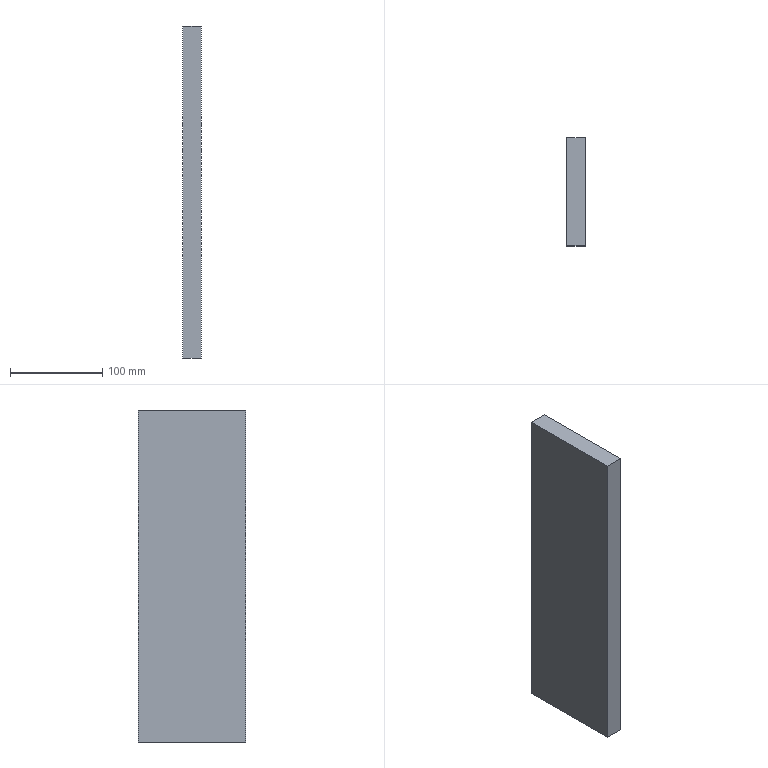Part | NX | features 底座(默认<按焊接>) 2 | 1 solid | 6 faces | box 20 x 116.68 x 360 mm | volume 840096 mm3 | plane 6
STEP:
#1=CARTESIAN_POINT('',(2704.525,684.,-26.));
#2=VERTEX_POINT('',#1);
#3=CARTESIAN_POINT('',(2704.525,567.32,-26.));
#4=VERTEX_POINT('',#3);
#5=CARTESIAN_POINT('',(2704.525,684.,-26.));
#6=DIRECTION('',(0.,-1.,0.));
#7=VECTOR('',#6,1000.);
#8=LINE('',#5,#7);
#9=EDGE_CURVE('',#2,#4,#8,.T.);
#10=ORIENTED_EDGE('',*,*,#9,.T.);
#11=CARTESIAN_POINT('',(2704.525,567.32,-386.));
#12=VERTEX_POINT('',#11);
#13=CARTESIAN_POINT('',(2704.525,567.32,-386.));
#14=DIRECTION('',(0.,0.,1.));
#15=VECTOR('',#14,1000.);
#16=LINE('',#13,#15);
#17=EDGE_CURVE('',#12,#4,#16,.T.);
#18=ORIENTED_EDGE('',*,*,#17,.F.);
#19=CARTESIAN_POINT('',(2704.525,684.,-386.));
#20=VERTEX_POINT('',#19);
#21=CARTESIAN_POINT('',(2704.525,684.,-386.));
#22=DIRECTION('',(0.,-1.,0.));
#23=VECTOR('',#22,1000.);
#24=LINE('',#21,#23);
#25=EDGE_CURVE('',#20,#12,#24,.T.);
#26=ORIENTED_EDGE('',*,*,#25,.F.);
#27=CARTESIAN_POINT('',(2704.525,684.,-386.));
#28=DIRECTION('',(0.,0.,1.));
#29=VECTOR('',#28,1000.);
#30=LINE('',#27,#29);
#31=EDGE_CURVE('',#20,#2,#30,.T.);
#32=ORIENTED_EDGE('',*,*,#31,.T.);
#33=EDGE_LOOP('',(#10,#18,#26,#32));
#34=FACE_BOUND('',#33,.T.);
#35=CARTESIAN_POINT('',(2704.525,684.,-386.));
#36=DIRECTION('',(-1.,0.,0.));
#37=DIRECTION('',(0.,0.,1.));
#38=AXIS2_PLACEMENT_3D('',#35,#36,#37);
#39=PLANE('',#38);
#40=ADVANCED_FACE('',(#34),#39,.F.);
#41=CARTESIAN_POINT('',(2684.525,567.32,-26.));
#42=VERTEX_POINT('',#41);
#43=CARTESIAN_POINT('',(2704.525,567.32,-26.));
#44=DIRECTION('',(-1.,0.,0.));
#45=VECTOR('',#44,1000.);
#46=LINE('',#43,#45);
#47=EDGE_CURVE('',#4,#42,#46,.T.);
#48=ORIENTED_EDGE('',*,*,#47,.T.);
#49=CARTESIAN_POINT('',(2684.525,567.32,-386.));
#50=VERTEX_POINT('',#49);
#51=CARTESIAN_POINT('',(2684.525,567.32,-386.));
#52=DIRECTION('',(0.,0.,1.));
#53=VECTOR('',#52,1000.);
#54=LINE('',#51,#53);
#55=EDGE_CURVE('',#50,#42,#54,.T.);
#56=ORIENTED_EDGE('',*,*,#55,.F.);
#57=CARTESIAN_POINT('',(2704.525,567.32,-386.));
#58=DIRECTION('',(-1.,0.,0.));
#59=VECTOR('',#58,1000.);
#60=LINE('',#57,#59);
#61=EDGE_CURVE('',#12,#50,#60,.T.);
#62=ORIENTED_EDGE('',*,*,#61,.F.);
#63=ORIENTED_EDGE('',*,*,#17,.T.);
#64=EDGE_LOOP('',(#48,#56,#62,#63));
#65=FACE_BOUND('',#64,.T.);
#66=CARTESIAN_POINT('',(2704.525,567.32,-386.));
#67=DIRECTION('',(0.,1.,0.));
#68=DIRECTION('',(0.,0.,1.));
#69=AXIS2_PLACEMENT_3D('',#66,#67,#68);
#70=PLANE('',#69);
#71=ADVANCED_FACE('',(#65),#70,.F.);
#72=CARTESIAN_POINT('',(2684.525,684.,-26.));
#73=VERTEX_POINT('',#72);
#74=CARTESIAN_POINT('',(2684.525,684.,-26.));
#75=DIRECTION('',(0.,1.,0.));
#76=VECTOR('',#75,1000.);
#77=LINE('',#74,#76);
#78=EDGE_CURVE('',#42,#73,#77,.T.);
#79=ORIENTED_EDGE('',*,*,#78,.T.);
#80=CARTESIAN_POINT('',(2684.525,684.,-386.));
#81=VERTEX_POINT('',#80);
#82=CARTESIAN_POINT('',(2684.525,684.,-386.));
#83=DIRECTION('',(0.,0.,1.));
#84=VECTOR('',#83,1000.);
#85=LINE('',#82,#84);
#86=EDGE_CURVE('',#81,#73,#85,.T.);
#87=ORIENTED_EDGE('',*,*,#86,.F.);
#88=CARTESIAN_POINT('',(2684.525,684.,-386.));
#89=DIRECTION('',(0.,1.,0.));
#90=VECTOR('',#89,1000.);
#91=LINE('',#88,#90);
#92=EDGE_CURVE('',#50,#81,#91,.T.);
#93=ORIENTED_EDGE('',*,*,#92,.F.);
#94=ORIENTED_EDGE('',*,*,#55,.T.);
#95=EDGE_LOOP('',(#79,#87,#93,#94));
#96=FACE_BOUND('',#95,.T.);
#97=CARTESIAN_POINT('',(2684.525,684.,-386.));
#98=DIRECTION('',(1.,0.,0.));
#99=DIRECTION('',(0.,0.,-1.));
#100=AXIS2_PLACEMENT_3D('',#97,#98,#99);
#101=PLANE('',#100);
#102=ADVANCED_FACE('',(#96),#101,.F.);
#103=CARTESIAN_POINT('',(2704.525,684.,-26.));
#104=DIRECTION('',(1.,0.,0.));
#105=VECTOR('',#104,1000.);
#106=LINE('',#103,#105);
#107=EDGE_CURVE('',#73,#2,#106,.T.);
#108=ORIENTED_EDGE('',*,*,#107,.T.);
#109=ORIENTED_EDGE('',*,*,#31,.F.);
#110=CARTESIAN_POINT('',(2704.525,684.,-386.));
#111=DIRECTION('',(1.,0.,0.));
#112=VECTOR('',#111,1000.);
#113=LINE('',#110,#112);
#114=EDGE_CURVE('',#81,#20,#113,.T.);
#115=ORIENTED_EDGE('',*,*,#114,.F.);
#116=ORIENTED_EDGE('',*,*,#86,.T.);
#117=EDGE_LOOP('',(#108,#109,#115,#116));
#118=FACE_BOUND('',#117,.T.);
#119=CARTESIAN_POINT('',(2704.525,684.,-386.));
#120=DIRECTION('',(0.,-1.,0.));
#121=DIRECTION('',(0.,0.,-1.));
#122=AXIS2_PLACEMENT_3D('',#119,#120,#121);
#123=PLANE('',#122);
#124=ADVANCED_FACE('',(#118),#123,.F.);
#125=ORIENTED_EDGE('',*,*,#25,.T.);
#126=ORIENTED_EDGE('',*,*,#61,.T.);
#127=ORIENTED_EDGE('',*,*,#92,.T.);
#128=ORIENTED_EDGE('',*,*,#114,.T.);
#129=EDGE_LOOP('',(#125,#126,#127,#128));
#130=FACE_BOUND('',#129,.T.);
#131=CARTESIAN_POINT('',(2704.525,567.32,-386.));
#132=DIRECTION('',(0.,0.,-1.));
#133=DIRECTION('',(-1.,0.,0.));
#134=AXIS2_PLACEMENT_3D('',#131,#132,#133);
#135=PLANE('',#134);
#136=ADVANCED_FACE('',(#130),#135,.T.);
#137=ORIENTED_EDGE('',*,*,#9,.F.);
#138=ORIENTED_EDGE('',*,*,#107,.F.);
#139=ORIENTED_EDGE('',*,*,#78,.F.);
#140=ORIENTED_EDGE('',*,*,#47,.F.);
#141=EDGE_LOOP('',(#137,#138,#139,#140));
#142=FACE_BOUND('',#141,.T.);
#143=CARTESIAN_POINT('',(2704.525,567.32,-26.));
#144=DIRECTION('',(0.,0.,-1.));
#145=DIRECTION('',(-1.,0.,0.));
#146=AXIS2_PLACEMENT_3D('',#143,#144,#145);
#147=PLANE('',#146);
#148=ADVANCED_FACE('',(#142),#147,.F.);
#149=CLOSED_SHELL('',(#40,#71,#102,#124,#136,#148));
#150=MANIFOLD_SOLID_BREP('',#149);
#151=(LENGTH_UNIT()NAMED_UNIT(*)SI_UNIT(.MILLI.,.METRE.));
#152=UNCERTAINTY_MEASURE_WITH_UNIT(LENGTH_MEASURE(0.00001),#151,'','');
#153=(NAMED_UNIT(*)PLANE_ANGLE_UNIT()SI_UNIT($,.RADIAN.));
#154=(NAMED_UNIT(*)SI_UNIT($,.STERADIAN.)SOLID_ANGLE_UNIT());
#155=(GEOMETRIC_REPRESENTATION_CONTEXT(3)GLOBAL_UNCERTAINTY_ASSIGNED_CONTEXT((#152))GLOBAL_UNIT_ASSIGNED_CONTEXT((#151,#153,#154))REPRESENTATION_CONTEXT('',''));
#156=ADVANCED_BREP_SHAPE_REPRESENTATION('',(#150),#155);